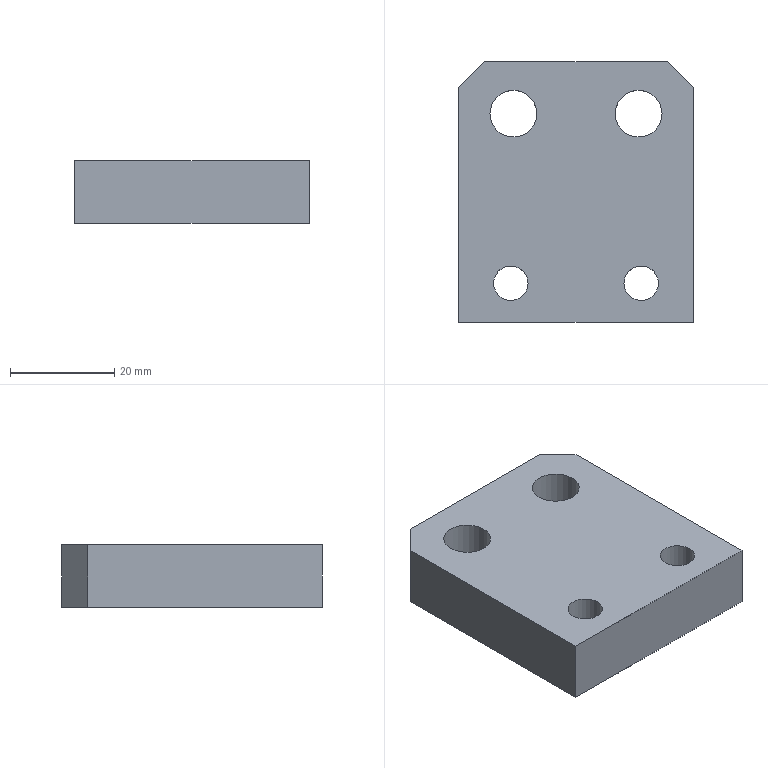Part | NX | 1 solid | 16 faces | box 45 x 50 x 12 mm | volume 23525 mm3 | plane 10 | cylinder 6 | commonest cylinder face diameters 6.6 x2 9 x2 11 x2
STEP:
#1=CARTESIAN_POINT('',(-22.5,30.,6.));
#2=VERTEX_POINT('',#1);
#3=CARTESIAN_POINT('',(-22.5,-15.,6.));
#4=VERTEX_POINT('',#3);
#5=CARTESIAN_POINT('',(-22.5,-15.,6.));
#6=DIRECTION('',(0.,-1.,0.));
#7=VECTOR('',#6,1000.);
#8=LINE('',#5,#7);
#9=EDGE_CURVE('',#2,#4,#8,.T.);
#10=ORIENTED_EDGE('',*,*,#9,.F.);
#11=CARTESIAN_POINT('',(-22.5,30.,-6.));
#12=VERTEX_POINT('',#11);
#13=CARTESIAN_POINT('',(-22.5,30.,6.));
#14=DIRECTION('',(0.,0.,-1.));
#15=VECTOR('',#14,1000.);
#16=LINE('',#13,#15);
#17=EDGE_CURVE('',#2,#12,#16,.T.);
#18=ORIENTED_EDGE('',*,*,#17,.T.);
#19=CARTESIAN_POINT('',(-22.5,-15.,-6.));
#20=VERTEX_POINT('',#19);
#21=CARTESIAN_POINT('',(-22.5,-15.,-6.));
#22=DIRECTION('',(0.,-1.,0.));
#23=VECTOR('',#22,1000.);
#24=LINE('',#21,#23);
#25=EDGE_CURVE('',#12,#20,#24,.T.);
#26=ORIENTED_EDGE('',*,*,#25,.T.);
#27=CARTESIAN_POINT('',(-22.5,-15.,6.));
#28=DIRECTION('',(0.,0.,-1.));
#29=VECTOR('',#28,1000.);
#30=LINE('',#27,#29);
#31=EDGE_CURVE('',#4,#20,#30,.T.);
#32=ORIENTED_EDGE('',*,*,#31,.F.);
#33=EDGE_LOOP('',(#10,#18,#26,#32));
#34=FACE_BOUND('',#33,.T.);
#35=CARTESIAN_POINT('',(-22.5,-15.,6.));
#36=DIRECTION('',(1.,0.,0.));
#37=DIRECTION('',(0.,0.,-1.));
#38=AXIS2_PLACEMENT_3D('',#35,#36,#37);
#39=PLANE('',#38);
#40=ADVANCED_FACE('',(#34),#39,.F.);
#41=CARTESIAN_POINT('',(22.5,-15.,-6.));
#42=VERTEX_POINT('',#41);
#43=CARTESIAN_POINT('',(22.5,-15.,-6.));
#44=DIRECTION('',(1.,0.,0.));
#45=VECTOR('',#44,1000.);
#46=LINE('',#43,#45);
#47=EDGE_CURVE('',#20,#42,#46,.T.);
#48=ORIENTED_EDGE('',*,*,#47,.T.);
#49=CARTESIAN_POINT('',(22.5,-15.,6.));
#50=VERTEX_POINT('',#49);
#51=CARTESIAN_POINT('',(22.5,-15.,6.));
#52=DIRECTION('',(0.,0.,-1.));
#53=VECTOR('',#52,1000.);
#54=LINE('',#51,#53);
#55=EDGE_CURVE('',#50,#42,#54,.T.);
#56=ORIENTED_EDGE('',*,*,#55,.F.);
#57=CARTESIAN_POINT('',(22.5,-15.,6.));
#58=DIRECTION('',(1.,0.,0.));
#59=VECTOR('',#58,1000.);
#60=LINE('',#57,#59);
#61=EDGE_CURVE('',#4,#50,#60,.T.);
#62=ORIENTED_EDGE('',*,*,#61,.F.);
#63=ORIENTED_EDGE('',*,*,#31,.T.);
#64=EDGE_LOOP('',(#48,#56,#62,#63));
#65=FACE_BOUND('',#64,.T.);
#66=CARTESIAN_POINT('',(22.5,-15.,6.));
#67=DIRECTION('',(0.,1.,0.));
#68=DIRECTION('',(-1.,0.,0.));
#69=AXIS2_PLACEMENT_3D('',#66,#67,#68);
#70=PLANE('',#69);
#71=ADVANCED_FACE('',(#65),#70,.F.);
#72=CARTESIAN_POINT('',(22.5,30.,-6.));
#73=VERTEX_POINT('',#72);
#74=CARTESIAN_POINT('',(22.5,35.,-6.));
#75=DIRECTION('',(0.,1.,0.));
#76=VECTOR('',#75,1000.);
#77=LINE('',#74,#76);
#78=EDGE_CURVE('',#42,#73,#77,.T.);
#79=ORIENTED_EDGE('',*,*,#78,.T.);
#80=CARTESIAN_POINT('',(22.5,30.,6.));
#81=VERTEX_POINT('',#80);
#82=CARTESIAN_POINT('',(22.5,30.,6.));
#83=DIRECTION('',(0.,0.,1.));
#84=VECTOR('',#83,1000.);
#85=LINE('',#82,#84);
#86=EDGE_CURVE('',#73,#81,#85,.T.);
#87=ORIENTED_EDGE('',*,*,#86,.T.);
#88=CARTESIAN_POINT('',(22.5,35.,6.));
#89=DIRECTION('',(0.,1.,0.));
#90=VECTOR('',#89,1000.);
#91=LINE('',#88,#90);
#92=EDGE_CURVE('',#50,#81,#91,.T.);
#93=ORIENTED_EDGE('',*,*,#92,.F.);
#94=ORIENTED_EDGE('',*,*,#55,.T.);
#95=EDGE_LOOP('',(#79,#87,#93,#94));
#96=FACE_BOUND('',#95,.T.);
#97=CARTESIAN_POINT('',(22.5,35.,6.));
#98=DIRECTION('',(-1.,0.,0.));
#99=DIRECTION('',(0.,-1.,0.));
#100=AXIS2_PLACEMENT_3D('',#97,#98,#99);
#101=PLANE('',#100);
#102=ADVANCED_FACE('',(#96),#101,.F.);
#103=CARTESIAN_POINT('',(17.5,35.,6.));
#104=VERTEX_POINT('',#103);
#105=CARTESIAN_POINT('',(-17.5,35.,6.));
#106=VERTEX_POINT('',#105);
#107=CARTESIAN_POINT('',(-22.5,35.,6.));
#108=DIRECTION('',(-1.,0.,0.));
#109=VECTOR('',#108,1000.);
#110=LINE('',#107,#109);
#111=EDGE_CURVE('',#104,#106,#110,.T.);
#112=ORIENTED_EDGE('',*,*,#111,.F.);
#113=CARTESIAN_POINT('',(17.5,35.,-6.));
#114=VERTEX_POINT('',#113);
#115=CARTESIAN_POINT('',(17.5,35.,6.));
#116=DIRECTION('',(0.,0.,-1.));
#117=VECTOR('',#116,1000.);
#118=LINE('',#115,#117);
#119=EDGE_CURVE('',#104,#114,#118,.T.);
#120=ORIENTED_EDGE('',*,*,#119,.T.);
#121=CARTESIAN_POINT('',(-17.5,35.,-6.));
#122=VERTEX_POINT('',#121);
#123=CARTESIAN_POINT('',(-22.5,35.,-6.));
#124=DIRECTION('',(-1.,0.,0.));
#125=VECTOR('',#124,1000.);
#126=LINE('',#123,#125);
#127=EDGE_CURVE('',#114,#122,#126,.T.);
#128=ORIENTED_EDGE('',*,*,#127,.T.);
#129=CARTESIAN_POINT('',(-17.5,35.,6.));
#130=DIRECTION('',(0.,0.,1.));
#131=VECTOR('',#130,1000.);
#132=LINE('',#129,#131);
#133=EDGE_CURVE('',#122,#106,#132,.T.);
#134=ORIENTED_EDGE('',*,*,#133,.T.);
#135=EDGE_LOOP('',(#112,#120,#128,#134));
#136=FACE_BOUND('',#135,.T.);
#137=CARTESIAN_POINT('',(-22.5,35.,6.));
#138=DIRECTION('',(0.,-1.,0.));
#139=DIRECTION('',(1.,0.,0.));
#140=AXIS2_PLACEMENT_3D('',#137,#138,#139);
#141=PLANE('',#140);
#142=ADVANCED_FACE('',(#136),#141,.F.);
#143=CARTESIAN_POINT('',(9.2,-7.5,6.));
#144=VERTEX_POINT('',#143);
#145=CARTESIAN_POINT('',(12.5,-7.5,6.));
#146=DIRECTION('',(0.,0.,-1.));
#147=DIRECTION('',(-1.,0.,0.));
#148=AXIS2_PLACEMENT_3D('',#145,#146,#147);
#149=CIRCLE('',#148,3.3);
#150=EDGE_CURVE('',#144,#144,#149,.T.);
#151=ORIENTED_EDGE('',*,*,#150,.T.);
#152=EDGE_LOOP('',(#151));
#153=FACE_BOUND('',#152,.T.);
#154=CARTESIAN_POINT('',(-15.8,-7.5,6.));
#155=VERTEX_POINT('',#154);
#156=CARTESIAN_POINT('',(-12.5,-7.5,6.));
#157=DIRECTION('',(0.,0.,-1.));
#158=DIRECTION('',(-1.,0.,0.));
#159=AXIS2_PLACEMENT_3D('',#156,#157,#158);
#160=CIRCLE('',#159,3.3);
#161=EDGE_CURVE('',#155,#155,#160,.T.);
#162=ORIENTED_EDGE('',*,*,#161,.T.);
#163=EDGE_LOOP('',(#162));
#164=FACE_BOUND('',#163,.T.);
#165=CARTESIAN_POINT('',(16.5,25.,6.));
#166=VERTEX_POINT('',#165);
#167=CARTESIAN_POINT('',(12.,25.,6.));
#168=DIRECTION('',(0.,0.,1.));
#169=DIRECTION('',(1.,0.,0.));
#170=AXIS2_PLACEMENT_3D('',#167,#168,#169);
#171=CIRCLE('',#170,4.5);
#172=EDGE_CURVE('',#166,#166,#171,.T.);
#173=ORIENTED_EDGE('',*,*,#172,.F.);
#174=EDGE_LOOP('',(#173));
#175=FACE_BOUND('',#174,.T.);
#176=CARTESIAN_POINT('',(-7.5,25.,6.));
#177=VERTEX_POINT('',#176);
#178=CARTESIAN_POINT('',(-12.,25.,6.));
#179=DIRECTION('',(0.,0.,1.));
#180=DIRECTION('',(1.,0.,0.));
#181=AXIS2_PLACEMENT_3D('',#178,#179,#180);
#182=CIRCLE('',#181,4.5);
#183=EDGE_CURVE('',#177,#177,#182,.T.);
#184=ORIENTED_EDGE('',*,*,#183,.F.);
#185=EDGE_LOOP('',(#184));
#186=FACE_BOUND('',#185,.T.);
#187=ORIENTED_EDGE('',*,*,#92,.T.);
#188=CARTESIAN_POINT('',(17.5,35.,6.));
#189=DIRECTION('',(0.7071,-0.7071,0.));
#190=VECTOR('',#189,1000.);
#191=LINE('',#188,#190);
#192=EDGE_CURVE('',#81,#104,#191,.F.);
#193=ORIENTED_EDGE('',*,*,#192,.T.);
#194=ORIENTED_EDGE('',*,*,#111,.T.);
#195=CARTESIAN_POINT('',(-22.5,30.,6.));
#196=DIRECTION('',(0.7071,0.7071,0.));
#197=VECTOR('',#196,1000.);
#198=LINE('',#195,#197);
#199=EDGE_CURVE('',#106,#2,#198,.F.);
#200=ORIENTED_EDGE('',*,*,#199,.T.);
#201=ORIENTED_EDGE('',*,*,#9,.T.);
#202=ORIENTED_EDGE('',*,*,#61,.T.);
#203=EDGE_LOOP('',(#187,#193,#194,#200,#201,#202));
#204=FACE_BOUND('',#203,.T.);
#205=CARTESIAN_POINT('',(0.,0.,6.));
#206=DIRECTION('',(0.,0.,-1.));
#207=DIRECTION('',(-1.,0.,0.));
#208=AXIS2_PLACEMENT_3D('',#205,#206,#207);
#209=PLANE('',#208);
#210=ADVANCED_FACE('',(#153,#164,#175,#186,#204),#209,.F.);
#211=CARTESIAN_POINT('',(7.,-7.5,-6.));
#212=VERTEX_POINT('',#211);
#213=CARTESIAN_POINT('',(12.5,-7.5,-6.));
#214=DIRECTION('',(0.,0.,-1.));
#215=DIRECTION('',(-1.,0.,0.));
#216=AXIS2_PLACEMENT_3D('',#213,#214,#215);
#217=CIRCLE('',#216,5.5);
#218=EDGE_CURVE('',#212,#212,#217,.T.);
#219=ORIENTED_EDGE('',*,*,#218,.F.);
#220=EDGE_LOOP('',(#219));
#221=FACE_BOUND('',#220,.T.);
#222=CARTESIAN_POINT('',(-18.,-7.5,-6.));
#223=VERTEX_POINT('',#222);
#224=CARTESIAN_POINT('',(-12.5,-7.5,-6.));
#225=DIRECTION('',(0.,0.,-1.));
#226=DIRECTION('',(-1.,0.,0.));
#227=AXIS2_PLACEMENT_3D('',#224,#225,#226);
#228=CIRCLE('',#227,5.5);
#229=EDGE_CURVE('',#223,#223,#228,.T.);
#230=ORIENTED_EDGE('',*,*,#229,.F.);
#231=EDGE_LOOP('',(#230));
#232=FACE_BOUND('',#231,.T.);
#233=CARTESIAN_POINT('',(16.5,25.,-6.));
#234=VERTEX_POINT('',#233);
#235=CARTESIAN_POINT('',(12.,25.,-6.));
#236=DIRECTION('',(0.,0.,1.));
#237=DIRECTION('',(1.,0.,0.));
#238=AXIS2_PLACEMENT_3D('',#235,#236,#237);
#239=CIRCLE('',#238,4.5);
#240=EDGE_CURVE('',#234,#234,#239,.T.);
#241=ORIENTED_EDGE('',*,*,#240,.T.);
#242=EDGE_LOOP('',(#241));
#243=FACE_BOUND('',#242,.T.);
#244=CARTESIAN_POINT('',(-7.5,25.,-6.));
#245=VERTEX_POINT('',#244);
#246=CARTESIAN_POINT('',(-12.,25.,-6.));
#247=DIRECTION('',(0.,0.,1.));
#248=DIRECTION('',(1.,0.,0.));
#249=AXIS2_PLACEMENT_3D('',#246,#247,#248);
#250=CIRCLE('',#249,4.5);
#251=EDGE_CURVE('',#245,#245,#250,.T.);
#252=ORIENTED_EDGE('',*,*,#251,.T.);
#253=EDGE_LOOP('',(#252));
#254=FACE_BOUND('',#253,.T.);
#255=ORIENTED_EDGE('',*,*,#127,.F.);
#256=CARTESIAN_POINT('',(26.25,26.25,-6.));
#257=DIRECTION('',(-0.7071,0.7071,0.));
#258=VECTOR('',#257,1000.);
#259=LINE('',#256,#258);
#260=EDGE_CURVE('',#114,#73,#259,.F.);
#261=ORIENTED_EDGE('',*,*,#260,.T.);
#262=ORIENTED_EDGE('',*,*,#78,.F.);
#263=ORIENTED_EDGE('',*,*,#47,.F.);
#264=ORIENTED_EDGE('',*,*,#25,.F.);
#265=CARTESIAN_POINT('',(-26.25,26.25,-6.));
#266=DIRECTION('',(-0.7071,-0.7071,0.));
#267=VECTOR('',#266,1000.);
#268=LINE('',#265,#267);
#269=EDGE_CURVE('',#12,#122,#268,.F.);
#270=ORIENTED_EDGE('',*,*,#269,.T.);
#271=EDGE_LOOP('',(#255,#261,#262,#263,#264,#270));
#272=FACE_BOUND('',#271,.T.);
#273=CARTESIAN_POINT('',(0.,0.,-6.));
#274=DIRECTION('',(0.,0.,-1.));
#275=DIRECTION('',(-1.,0.,0.));
#276=AXIS2_PLACEMENT_3D('',#273,#274,#275);
#277=PLANE('',#276);
#278=ADVANCED_FACE('',(#221,#232,#243,#254,#272),#277,.T.);
#279=ORIENTED_EDGE('',*,*,#192,.F.);
#280=ORIENTED_EDGE('',*,*,#86,.F.);
#281=ORIENTED_EDGE('',*,*,#260,.F.);
#282=ORIENTED_EDGE('',*,*,#119,.F.);
#283=EDGE_LOOP('',(#279,#280,#281,#282));
#284=FACE_BOUND('',#283,.T.);
#285=CARTESIAN_POINT('',(17.5,35.,6.));
#286=DIRECTION('',(-0.7071,-0.7071,0.));
#287=DIRECTION('',(0.,0.,-1.));
#288=AXIS2_PLACEMENT_3D('',#285,#286,#287);
#289=PLANE('',#288);
#290=ADVANCED_FACE('',(#284),#289,.F.);
#291=ORIENTED_EDGE('',*,*,#199,.F.);
#292=ORIENTED_EDGE('',*,*,#133,.F.);
#293=ORIENTED_EDGE('',*,*,#269,.F.);
#294=ORIENTED_EDGE('',*,*,#17,.F.);
#295=EDGE_LOOP('',(#291,#292,#293,#294));
#296=FACE_BOUND('',#295,.T.);
#297=CARTESIAN_POINT('',(-22.5,30.,6.));
#298=DIRECTION('',(0.7071,-0.7071,0.));
#299=DIRECTION('',(0.,0.,-1.));
#300=AXIS2_PLACEMENT_3D('',#297,#298,#299);
#301=PLANE('',#300);
#302=ADVANCED_FACE('',(#296),#301,.F.);
#303=ORIENTED_EDGE('',*,*,#251,.F.);
#304=EDGE_LOOP('',(#303));
#305=FACE_BOUND('',#304,.T.);
#306=ORIENTED_EDGE('',*,*,#183,.T.);
#307=EDGE_LOOP('',(#306));
#308=FACE_BOUND('',#307,.T.);
#309=CARTESIAN_POINT('',(-12.,25.,6.));
#310=DIRECTION('',(0.,0.,1.));
#311=DIRECTION('',(1.,0.,0.));
#312=AXIS2_PLACEMENT_3D('',#309,#310,#311);
#313=CYLINDRICAL_SURFACE('',#312,4.5);
#314=ADVANCED_FACE('',(#305,#308),#313,.F.);
#315=ORIENTED_EDGE('',*,*,#240,.F.);
#316=EDGE_LOOP('',(#315));
#317=FACE_BOUND('',#316,.T.);
#318=ORIENTED_EDGE('',*,*,#172,.T.);
#319=EDGE_LOOP('',(#318));
#320=FACE_BOUND('',#319,.T.);
#321=CARTESIAN_POINT('',(12.,25.,6.));
#322=DIRECTION('',(0.,0.,1.));
#323=DIRECTION('',(1.,0.,0.));
#324=AXIS2_PLACEMENT_3D('',#321,#322,#323);
#325=CYLINDRICAL_SURFACE('',#324,4.5);
#326=ADVANCED_FACE('',(#317,#320),#325,.F.);
#327=ORIENTED_EDGE('',*,*,#161,.F.);
#328=EDGE_LOOP('',(#327));
#329=FACE_BOUND('',#328,.T.);
#330=CARTESIAN_POINT('',(-15.8,-7.5,0.8));
#331=VERTEX_POINT('',#330);
#332=CARTESIAN_POINT('',(-12.5,-7.5,0.8));
#333=DIRECTION('',(0.,0.,-1.));
#334=DIRECTION('',(-1.,0.,0.));
#335=AXIS2_PLACEMENT_3D('',#332,#333,#334);
#336=CIRCLE('',#335,3.3);
#337=EDGE_CURVE('',#331,#331,#336,.T.);
#338=ORIENTED_EDGE('',*,*,#337,.T.);
#339=EDGE_LOOP('',(#338));
#340=FACE_BOUND('',#339,.T.);
#341=CARTESIAN_POINT('',(-12.5,-7.5,-6.));
#342=DIRECTION('',(0.,0.,-1.));
#343=DIRECTION('',(-1.,0.,0.));
#344=AXIS2_PLACEMENT_3D('',#341,#342,#343);
#345=CYLINDRICAL_SURFACE('',#344,3.3);
#346=ADVANCED_FACE('',(#329,#340),#345,.F.);
#347=ORIENTED_EDGE('',*,*,#337,.F.);
#348=EDGE_LOOP('',(#347));
#349=FACE_BOUND('',#348,.T.);
#350=CARTESIAN_POINT('',(-18.,-7.5,0.8));
#351=VERTEX_POINT('',#350);
#352=CARTESIAN_POINT('',(-12.5,-7.5,0.8));
#353=DIRECTION('',(0.,0.,-1.));
#354=DIRECTION('',(-1.,0.,0.));
#355=AXIS2_PLACEMENT_3D('',#352,#353,#354);
#356=CIRCLE('',#355,5.5);
#357=EDGE_CURVE('',#351,#351,#356,.T.);
#358=ORIENTED_EDGE('',*,*,#357,.T.);
#359=EDGE_LOOP('',(#358));
#360=FACE_BOUND('',#359,.T.);
#361=CARTESIAN_POINT('',(-9.2,-7.5,0.8));
#362=DIRECTION('',(0.,0.,1.));
#363=DIRECTION('',(1.,0.,0.));
#364=AXIS2_PLACEMENT_3D('',#361,#362,#363);
#365=PLANE('',#364);
#366=ADVANCED_FACE('',(#349,#360),#365,.F.);
#367=ORIENTED_EDGE('',*,*,#357,.F.);
#368=EDGE_LOOP('',(#367));
#369=FACE_BOUND('',#368,.T.);
#370=ORIENTED_EDGE('',*,*,#229,.T.);
#371=EDGE_LOOP('',(#370));
#372=FACE_BOUND('',#371,.T.);
#373=CARTESIAN_POINT('',(-12.5,-7.5,-6.));
#374=DIRECTION('',(0.,0.,-1.));
#375=DIRECTION('',(-1.,0.,0.));
#376=AXIS2_PLACEMENT_3D('',#373,#374,#375);
#377=CYLINDRICAL_SURFACE('',#376,5.5);
#378=ADVANCED_FACE('',(#369,#372),#377,.F.);
#379=ORIENTED_EDGE('',*,*,#150,.F.);
#380=EDGE_LOOP('',(#379));
#381=FACE_BOUND('',#380,.T.);
#382=CARTESIAN_POINT('',(9.2,-7.5,0.8));
#383=VERTEX_POINT('',#382);
#384=CARTESIAN_POINT('',(12.5,-7.5,0.8));
#385=DIRECTION('',(0.,0.,-1.));
#386=DIRECTION('',(-1.,0.,0.));
#387=AXIS2_PLACEMENT_3D('',#384,#385,#386);
#388=CIRCLE('',#387,3.3);
#389=EDGE_CURVE('',#383,#383,#388,.T.);
#390=ORIENTED_EDGE('',*,*,#389,.T.);
#391=EDGE_LOOP('',(#390));
#392=FACE_BOUND('',#391,.T.);
#393=CARTESIAN_POINT('',(12.5,-7.5,-6.));
#394=DIRECTION('',(0.,0.,-1.));
#395=DIRECTION('',(-1.,0.,0.));
#396=AXIS2_PLACEMENT_3D('',#393,#394,#395);
#397=CYLINDRICAL_SURFACE('',#396,3.3);
#398=ADVANCED_FACE('',(#381,#392),#397,.F.);
#399=ORIENTED_EDGE('',*,*,#389,.F.);
#400=EDGE_LOOP('',(#399));
#401=FACE_BOUND('',#400,.T.);
#402=CARTESIAN_POINT('',(7.,-7.5,0.8));
#403=VERTEX_POINT('',#402);
#404=CARTESIAN_POINT('',(12.5,-7.5,0.8));
#405=DIRECTION('',(0.,0.,-1.));
#406=DIRECTION('',(-1.,0.,0.));
#407=AXIS2_PLACEMENT_3D('',#404,#405,#406);
#408=CIRCLE('',#407,5.5);
#409=EDGE_CURVE('',#403,#403,#408,.T.);
#410=ORIENTED_EDGE('',*,*,#409,.T.);
#411=EDGE_LOOP('',(#410));
#412=FACE_BOUND('',#411,.T.);
#413=CARTESIAN_POINT('',(15.8,-7.5,0.8));
#414=DIRECTION('',(0.,0.,1.));
#415=DIRECTION('',(1.,0.,0.));
#416=AXIS2_PLACEMENT_3D('',#413,#414,#415);
#417=PLANE('',#416);
#418=ADVANCED_FACE('',(#401,#412),#417,.F.);
#419=ORIENTED_EDGE('',*,*,#409,.F.);
#420=EDGE_LOOP('',(#419));
#421=FACE_BOUND('',#420,.T.);
#422=ORIENTED_EDGE('',*,*,#218,.T.);
#423=EDGE_LOOP('',(#422));
#424=FACE_BOUND('',#423,.T.);
#425=CARTESIAN_POINT('',(12.5,-7.5,-6.));
#426=DIRECTION('',(0.,0.,-1.));
#427=DIRECTION('',(-1.,0.,0.));
#428=AXIS2_PLACEMENT_3D('',#425,#426,#427);
#429=CYLINDRICAL_SURFACE('',#428,5.5);
#430=ADVANCED_FACE('',(#421,#424),#429,.F.);
#431=CLOSED_SHELL('',(#40,#71,#102,#142,#210,#278,#290,#302,#314,#326,#346,#366,#378,#398,#418,#430));
#432=MANIFOLD_SOLID_BREP('',#431);
#433=(LENGTH_UNIT()NAMED_UNIT(*)SI_UNIT(.MILLI.,.METRE.));
#434=UNCERTAINTY_MEASURE_WITH_UNIT(LENGTH_MEASURE(0.00001),#433,'','');
#435=(NAMED_UNIT(*)PLANE_ANGLE_UNIT()SI_UNIT($,.RADIAN.));
#436=(NAMED_UNIT(*)SI_UNIT($,.STERADIAN.)SOLID_ANGLE_UNIT());
#437=(GEOMETRIC_REPRESENTATION_CONTEXT(3)GLOBAL_UNCERTAINTY_ASSIGNED_CONTEXT((#434))GLOBAL_UNIT_ASSIGNED_CONTEXT((#433,#435,#436))REPRESENTATION_CONTEXT('',''));
#438=ADVANCED_BREP_SHAPE_REPRESENTATION('',(#432),#437);